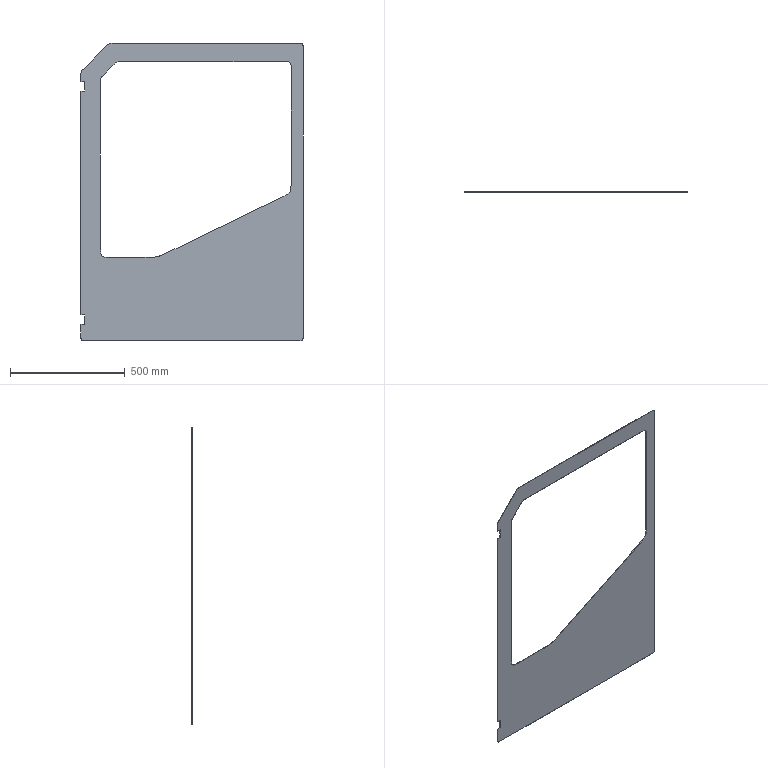Part | NX | features BREP 1 | 1 solid | 35 faces | box 967.789 x 12 x 1295 mm | volume 1241371 mm3 | plane 24 | spline 11